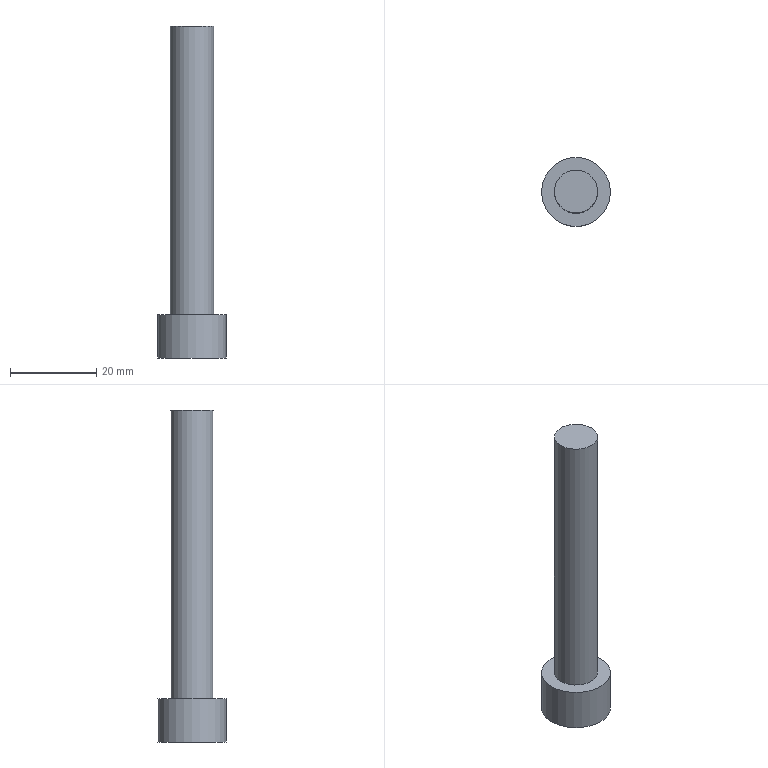Part | NX | features solid 2 | 1 solid | 12 faces | box 16 x 16 x 77 mm | volume 6996 mm3 | plane 10 | cylinder 2 | commonest cylinder face diameters 10 x1 16 x1
STEP:
#1=CARTESIAN_POINT('',(845.,40.,270.));
#2=VERTEX_POINT('',#1);
#3=CARTESIAN_POINT('',(850.,40.,270.));
#4=DIRECTION('',(0.,0.,-1.));
#5=DIRECTION('',(-1.,0.,0.));
#6=AXIS2_PLACEMENT_3D('',#3,#4,#5);
#7=CIRCLE('',#6,5.);
#8=EDGE_CURVE('',#2,#2,#7,.T.);
#9=ORIENTED_EDGE('',*,*,#8,.F.);
#10=EDGE_LOOP('',(#9));
#11=FACE_BOUND('',#10,.T.);
#12=CARTESIAN_POINT('',(845.,40.,337.));
#13=VERTEX_POINT('',#12);
#14=CARTESIAN_POINT('',(850.,40.,337.));
#15=DIRECTION('',(0.,0.,-1.));
#16=DIRECTION('',(-1.,0.,0.));
#17=AXIS2_PLACEMENT_3D('',#14,#15,#16);
#18=CIRCLE('',#17,5.);
#19=EDGE_CURVE('',#13,#13,#18,.T.);
#20=ORIENTED_EDGE('',*,*,#19,.T.);
#21=EDGE_LOOP('',(#20));
#22=FACE_BOUND('',#21,.T.);
#23=CARTESIAN_POINT('',(850.,40.,337.));
#24=DIRECTION('',(0.,0.,-1.));
#25=DIRECTION('',(1.,0.,0.));
#26=AXIS2_PLACEMENT_3D('',#23,#24,#25);
#27=CYLINDRICAL_SURFACE('',#26,5.);
#28=ADVANCED_FACE('',(#11,#22),#27,.T.);
#29=ORIENTED_EDGE('',*,*,#19,.F.);
#30=EDGE_LOOP('',(#29));
#31=FACE_BOUND('',#30,.T.);
#32=CARTESIAN_POINT('',(850.,40.,337.));
#33=DIRECTION('',(0.,0.,1.));
#34=DIRECTION('',(-1.,0.,0.));
#35=AXIS2_PLACEMENT_3D('',#32,#33,#34);
#36=PLANE('',#35);
#37=ADVANCED_FACE('',(#31),#36,.T.);
#38=CARTESIAN_POINT('',(842.,40.,270.));
#39=VERTEX_POINT('',#38);
#40=CARTESIAN_POINT('',(850.,40.,270.));
#41=DIRECTION('',(0.,0.,-1.));
#42=DIRECTION('',(-1.,0.,0.));
#43=AXIS2_PLACEMENT_3D('',#40,#41,#42);
#44=CIRCLE('',#43,8.);
#45=EDGE_CURVE('',#39,#39,#44,.T.);
#46=ORIENTED_EDGE('',*,*,#45,.F.);
#47=EDGE_LOOP('',(#46));
#48=FACE_BOUND('',#47,.T.);
#49=ORIENTED_EDGE('',*,*,#8,.T.);
#50=EDGE_LOOP('',(#49));
#51=FACE_BOUND('',#50,.T.);
#52=CARTESIAN_POINT('',(850.,40.,270.));
#53=DIRECTION('',(0.,0.,1.));
#54=DIRECTION('',(-1.,0.,0.));
#55=AXIS2_PLACEMENT_3D('',#52,#53,#54);
#56=PLANE('',#55);
#57=ADVANCED_FACE('',(#48,#51),#56,.T.);
#58=CARTESIAN_POINT('',(842.,40.,260.));
#59=VERTEX_POINT('',#58);
#60=CARTESIAN_POINT('',(850.,40.,260.));
#61=DIRECTION('',(0.,0.,-1.));
#62=DIRECTION('',(-1.,0.,0.));
#63=AXIS2_PLACEMENT_3D('',#60,#61,#62);
#64=CIRCLE('',#63,8.);
#65=EDGE_CURVE('',#59,#59,#64,.T.);
#66=ORIENTED_EDGE('',*,*,#65,.F.);
#67=EDGE_LOOP('',(#66));
#68=FACE_BOUND('',#67,.T.);
#69=ORIENTED_EDGE('',*,*,#45,.T.);
#70=EDGE_LOOP('',(#69));
#71=FACE_BOUND('',#70,.T.);
#72=CARTESIAN_POINT('',(850.,40.,260.));
#73=DIRECTION('',(0.,0.,1.));
#74=DIRECTION('',(-1.,0.,0.));
#75=AXIS2_PLACEMENT_3D('',#72,#73,#74);
#76=CYLINDRICAL_SURFACE('',#75,8.);
#77=ADVANCED_FACE('',(#68,#71),#76,.T.);
#78=CARTESIAN_POINT('',(846.,42.309,260.));
#79=VERTEX_POINT('',#78);
#80=CARTESIAN_POINT('',(850.,44.619,260.));
#81=VERTEX_POINT('',#80);
#82=CARTESIAN_POINT('',(848.,43.464,260.));
#83=DIRECTION('',(0.866,0.5,0.));
#84=VECTOR('',#83,1000.);
#85=LINE('',#82,#84);
#86=EDGE_CURVE('',#79,#81,#85,.T.);
#87=ORIENTED_EDGE('',*,*,#86,.F.);
#88=CARTESIAN_POINT('',(846.,37.691,260.));
#89=VERTEX_POINT('',#88);
#90=CARTESIAN_POINT('',(846.,40.,260.));
#91=DIRECTION('',(0.,1.,0.));
#92=VECTOR('',#91,1000.);
#93=LINE('',#90,#92);
#94=EDGE_CURVE('',#89,#79,#93,.T.);
#95=ORIENTED_EDGE('',*,*,#94,.F.);
#96=CARTESIAN_POINT('',(850.,35.381,260.));
#97=VERTEX_POINT('',#96);
#98=CARTESIAN_POINT('',(848.,36.536,260.));
#99=DIRECTION('',(-0.866,0.5,0.));
#100=VECTOR('',#99,1000.);
#101=LINE('',#98,#100);
#102=EDGE_CURVE('',#97,#89,#101,.T.);
#103=ORIENTED_EDGE('',*,*,#102,.F.);
#104=CARTESIAN_POINT('',(854.,37.691,260.));
#105=VERTEX_POINT('',#104);
#106=CARTESIAN_POINT('',(852.,36.536,260.));
#107=DIRECTION('',(-0.866,-0.5,0.));
#108=VECTOR('',#107,1000.);
#109=LINE('',#106,#108);
#110=EDGE_CURVE('',#105,#97,#109,.T.);
#111=ORIENTED_EDGE('',*,*,#110,.F.);
#112=CARTESIAN_POINT('',(854.,42.309,260.));
#113=VERTEX_POINT('',#112);
#114=CARTESIAN_POINT('',(854.,40.,260.));
#115=DIRECTION('',(0.,-1.,0.));
#116=VECTOR('',#115,1000.);
#117=LINE('',#114,#116);
#118=EDGE_CURVE('',#113,#105,#117,.T.);
#119=ORIENTED_EDGE('',*,*,#118,.F.);
#120=CARTESIAN_POINT('',(852.,43.464,260.));
#121=DIRECTION('',(0.866,-0.5,0.));
#122=VECTOR('',#121,1000.);
#123=LINE('',#120,#122);
#124=EDGE_CURVE('',#81,#113,#123,.T.);
#125=ORIENTED_EDGE('',*,*,#124,.F.);
#126=EDGE_LOOP('',(#87,#95,#103,#111,#119,#125));
#127=FACE_BOUND('',#126,.T.);
#128=ORIENTED_EDGE('',*,*,#65,.T.);
#129=EDGE_LOOP('',(#128));
#130=FACE_BOUND('',#129,.T.);
#131=CARTESIAN_POINT('',(850.,40.,260.));
#132=DIRECTION('',(0.,0.,1.));
#133=DIRECTION('',(-1.,0.,0.));
#134=AXIS2_PLACEMENT_3D('',#131,#132,#133);
#135=PLANE('',#134);
#136=ADVANCED_FACE('',(#127,#130),#135,.F.);
#137=CARTESIAN_POINT('',(850.,44.619,265.));
#138=VERTEX_POINT('',#137);
#139=CARTESIAN_POINT('',(850.,44.619,245.));
#140=DIRECTION('',(0.,0.,1.));
#141=VECTOR('',#140,1000.);
#142=LINE('',#139,#141);
#143=EDGE_CURVE('',#81,#138,#142,.T.);
#144=ORIENTED_EDGE('',*,*,#143,.F.);
#145=ORIENTED_EDGE('',*,*,#124,.T.);
#146=CARTESIAN_POINT('',(854.,42.309,265.));
#147=VERTEX_POINT('',#146);
#148=CARTESIAN_POINT('',(854.,42.309,245.));
#149=DIRECTION('',(0.,0.,1.));
#150=VECTOR('',#149,1000.);
#151=LINE('',#148,#150);
#152=EDGE_CURVE('',#113,#147,#151,.T.);
#153=ORIENTED_EDGE('',*,*,#152,.T.);
#154=CARTESIAN_POINT('',(850.,44.619,265.));
#155=DIRECTION('',(0.866,-0.5,0.));
#156=VECTOR('',#155,1000.);
#157=LINE('',#154,#156);
#158=EDGE_CURVE('',#138,#147,#157,.T.);
#159=ORIENTED_EDGE('',*,*,#158,.F.);
#160=EDGE_LOOP('',(#144,#145,#153,#159));
#161=FACE_BOUND('',#160,.T.);
#162=CARTESIAN_POINT('',(850.,44.619,245.));
#163=DIRECTION('',(0.5,0.866,0.));
#164=DIRECTION('',(0.866,-0.5,0.));
#165=AXIS2_PLACEMENT_3D('',#162,#163,#164);
#166=PLANE('',#165);
#167=ADVANCED_FACE('',(#161),#166,.F.);
#168=ORIENTED_EDGE('',*,*,#152,.F.);
#169=ORIENTED_EDGE('',*,*,#118,.T.);
#170=CARTESIAN_POINT('',(854.,37.691,265.));
#171=VERTEX_POINT('',#170);
#172=CARTESIAN_POINT('',(854.,37.691,245.));
#173=DIRECTION('',(0.,0.,1.));
#174=VECTOR('',#173,1000.);
#175=LINE('',#172,#174);
#176=EDGE_CURVE('',#105,#171,#175,.T.);
#177=ORIENTED_EDGE('',*,*,#176,.T.);
#178=CARTESIAN_POINT('',(854.,42.309,265.));
#179=DIRECTION('',(0.,-1.,0.));
#180=VECTOR('',#179,1000.);
#181=LINE('',#178,#180);
#182=EDGE_CURVE('',#147,#171,#181,.T.);
#183=ORIENTED_EDGE('',*,*,#182,.F.);
#184=EDGE_LOOP('',(#168,#169,#177,#183));
#185=FACE_BOUND('',#184,.T.);
#186=CARTESIAN_POINT('',(854.,42.309,245.));
#187=DIRECTION('',(1.,0.,0.));
#188=DIRECTION('',(0.,0.,1.));
#189=AXIS2_PLACEMENT_3D('',#186,#187,#188);
#190=PLANE('',#189);
#191=ADVANCED_FACE('',(#185),#190,.F.);
#192=ORIENTED_EDGE('',*,*,#176,.F.);
#193=ORIENTED_EDGE('',*,*,#110,.T.);
#194=CARTESIAN_POINT('',(850.,35.381,265.));
#195=VERTEX_POINT('',#194);
#196=CARTESIAN_POINT('',(850.,35.381,245.));
#197=DIRECTION('',(0.,0.,1.));
#198=VECTOR('',#197,1000.);
#199=LINE('',#196,#198);
#200=EDGE_CURVE('',#97,#195,#199,.T.);
#201=ORIENTED_EDGE('',*,*,#200,.T.);
#202=CARTESIAN_POINT('',(854.,37.691,265.));
#203=DIRECTION('',(-0.866,-0.5,0.));
#204=VECTOR('',#203,1000.);
#205=LINE('',#202,#204);
#206=EDGE_CURVE('',#171,#195,#205,.T.);
#207=ORIENTED_EDGE('',*,*,#206,.F.);
#208=EDGE_LOOP('',(#192,#193,#201,#207));
#209=FACE_BOUND('',#208,.T.);
#210=CARTESIAN_POINT('',(854.,37.691,245.));
#211=DIRECTION('',(0.5,-0.866,0.));
#212=DIRECTION('',(-0.866,-0.5,0.));
#213=AXIS2_PLACEMENT_3D('',#210,#211,#212);
#214=PLANE('',#213);
#215=ADVANCED_FACE('',(#209),#214,.F.);
#216=ORIENTED_EDGE('',*,*,#200,.F.);
#217=ORIENTED_EDGE('',*,*,#102,.T.);
#218=CARTESIAN_POINT('',(846.,37.691,265.));
#219=VERTEX_POINT('',#218);
#220=CARTESIAN_POINT('',(846.,37.691,245.));
#221=DIRECTION('',(0.,0.,1.));
#222=VECTOR('',#221,1000.);
#223=LINE('',#220,#222);
#224=EDGE_CURVE('',#89,#219,#223,.T.);
#225=ORIENTED_EDGE('',*,*,#224,.T.);
#226=CARTESIAN_POINT('',(850.,35.381,265.));
#227=DIRECTION('',(-0.866,0.5,0.));
#228=VECTOR('',#227,1000.);
#229=LINE('',#226,#228);
#230=EDGE_CURVE('',#195,#219,#229,.T.);
#231=ORIENTED_EDGE('',*,*,#230,.F.);
#232=EDGE_LOOP('',(#216,#217,#225,#231));
#233=FACE_BOUND('',#232,.T.);
#234=CARTESIAN_POINT('',(850.,35.381,245.));
#235=DIRECTION('',(-0.5,-0.866,0.));
#236=DIRECTION('',(-0.866,0.5,0.));
#237=AXIS2_PLACEMENT_3D('',#234,#235,#236);
#238=PLANE('',#237);
#239=ADVANCED_FACE('',(#233),#238,.F.);
#240=ORIENTED_EDGE('',*,*,#224,.F.);
#241=ORIENTED_EDGE('',*,*,#94,.T.);
#242=CARTESIAN_POINT('',(846.,42.309,265.));
#243=VERTEX_POINT('',#242);
#244=CARTESIAN_POINT('',(846.,42.309,245.));
#245=DIRECTION('',(0.,0.,1.));
#246=VECTOR('',#245,1000.);
#247=LINE('',#244,#246);
#248=EDGE_CURVE('',#79,#243,#247,.T.);
#249=ORIENTED_EDGE('',*,*,#248,.T.);
#250=CARTESIAN_POINT('',(846.,37.691,265.));
#251=DIRECTION('',(0.,1.,0.));
#252=VECTOR('',#251,1000.);
#253=LINE('',#250,#252);
#254=EDGE_CURVE('',#219,#243,#253,.T.);
#255=ORIENTED_EDGE('',*,*,#254,.F.);
#256=EDGE_LOOP('',(#240,#241,#249,#255));
#257=FACE_BOUND('',#256,.T.);
#258=CARTESIAN_POINT('',(846.,37.691,245.));
#259=DIRECTION('',(-1.,0.,0.));
#260=DIRECTION('',(0.,0.,-1.));
#261=AXIS2_PLACEMENT_3D('',#258,#259,#260);
#262=PLANE('',#261);
#263=ADVANCED_FACE('',(#257),#262,.F.);
#264=ORIENTED_EDGE('',*,*,#248,.F.);
#265=ORIENTED_EDGE('',*,*,#86,.T.);
#266=ORIENTED_EDGE('',*,*,#143,.T.);
#267=CARTESIAN_POINT('',(846.,42.309,265.));
#268=DIRECTION('',(0.866,0.5,0.));
#269=VECTOR('',#268,1000.);
#270=LINE('',#267,#269);
#271=EDGE_CURVE('',#243,#138,#270,.T.);
#272=ORIENTED_EDGE('',*,*,#271,.F.);
#273=EDGE_LOOP('',(#264,#265,#266,#272));
#274=FACE_BOUND('',#273,.T.);
#275=CARTESIAN_POINT('',(846.,42.309,245.));
#276=DIRECTION('',(-0.5,0.866,0.));
#277=DIRECTION('',(0.866,0.5,0.));
#278=AXIS2_PLACEMENT_3D('',#275,#276,#277);
#279=PLANE('',#278);
#280=ADVANCED_FACE('',(#274),#279,.F.);
#281=ORIENTED_EDGE('',*,*,#158,.T.);
#282=ORIENTED_EDGE('',*,*,#182,.T.);
#283=ORIENTED_EDGE('',*,*,#206,.T.);
#284=ORIENTED_EDGE('',*,*,#230,.T.);
#285=ORIENTED_EDGE('',*,*,#254,.T.);
#286=ORIENTED_EDGE('',*,*,#271,.T.);
#287=EDGE_LOOP('',(#281,#282,#283,#284,#285,#286));
#288=FACE_BOUND('',#287,.T.);
#289=CARTESIAN_POINT('',(858.,40.,265.));
#290=DIRECTION('',(0.,0.,1.));
#291=DIRECTION('',(-1.,0.,0.));
#292=AXIS2_PLACEMENT_3D('',#289,#290,#291);
#293=PLANE('',#292);
#294=ADVANCED_FACE('',(#288),#293,.F.);
#295=CLOSED_SHELL('',(#28,#37,#57,#77,#136,#167,#191,#215,#239,#263,#280,#294));
#296=MANIFOLD_SOLID_BREP('',#295);
#297=(LENGTH_UNIT()NAMED_UNIT(*)SI_UNIT(.MILLI.,.METRE.));
#298=UNCERTAINTY_MEASURE_WITH_UNIT(LENGTH_MEASURE(0.00001),#297,'','');
#299=(NAMED_UNIT(*)PLANE_ANGLE_UNIT()SI_UNIT($,.RADIAN.));
#300=(NAMED_UNIT(*)SI_UNIT($,.STERADIAN.)SOLID_ANGLE_UNIT());
#301=(GEOMETRIC_REPRESENTATION_CONTEXT(3)GLOBAL_UNCERTAINTY_ASSIGNED_CONTEXT((#298))GLOBAL_UNIT_ASSIGNED_CONTEXT((#297,#299,#300))REPRESENTATION_CONTEXT('',''));
#302=ADVANCED_BREP_SHAPE_REPRESENTATION('',(#296),#301);